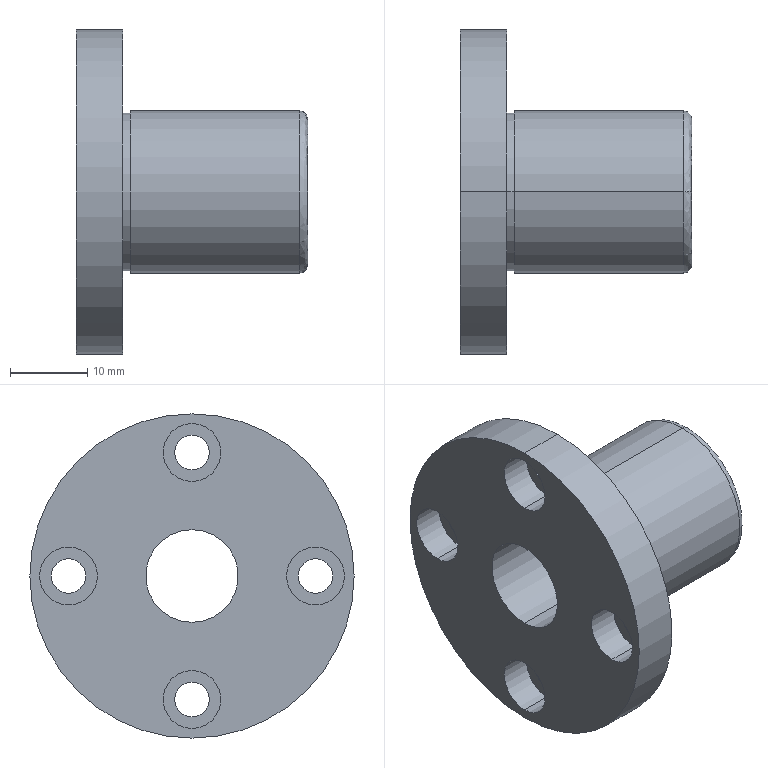Part | STEP file | LHFR122_Default | 1 solid | 34 faces | box 30 x 42 x 42 mm | volume 12352 mm3 | cylinder 24 | plane 7 | spline 3 | commonest cylinder face diameters 4.5 x8 7.5 x8 12 x2 20.4 x2 21 x2 42 x2